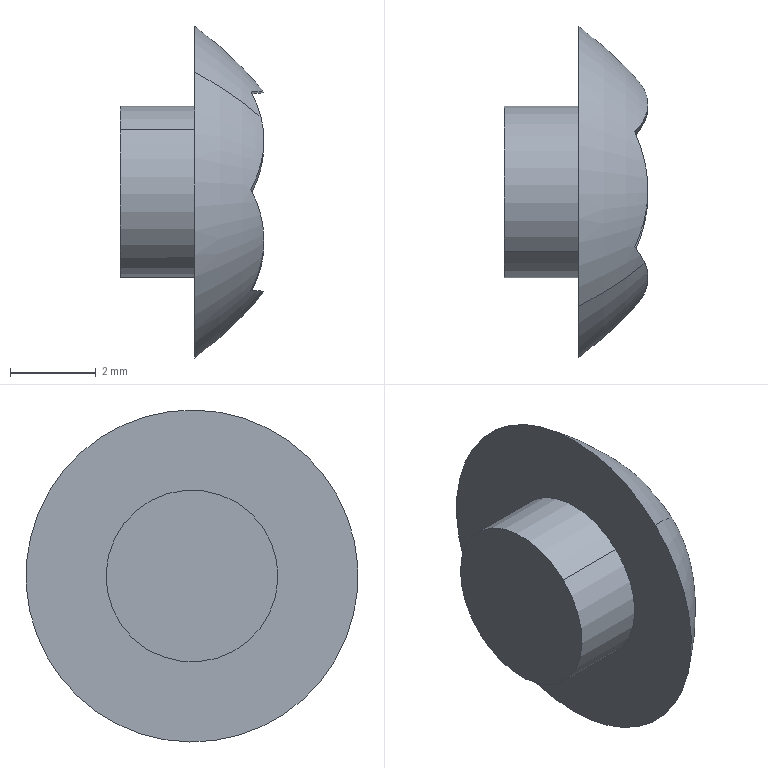Part | STEP file | OBJECT_38-2315 | 1 solid | 13 faces | box 3.344 x 7.727 x 7.727 mm | volume 53.316 mm3 | plane 9 | cylinder 2 | other 2 | commonest cylinder face diameters 4 x2